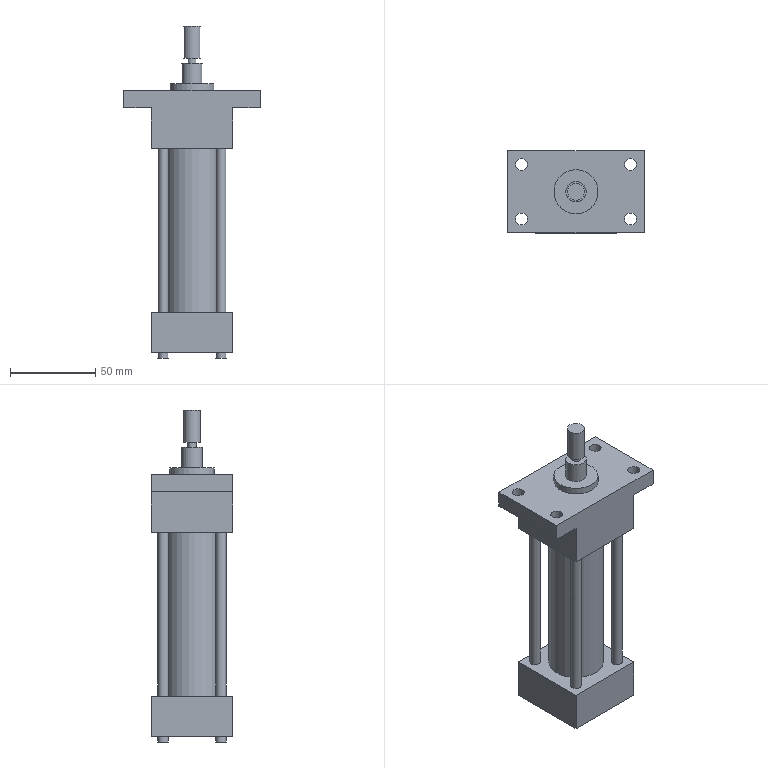Part | NX | features solid 2 | 1 solid | 48 faces | box 80 x 48 x 195 mm | volume 184667 mm3 | plane 28 | cylinder 20 | commonest cylinder face diameters 6 x8 7 x4 10 x3 5 x1 12 x1 26 x1
STEP:
#1=CARTESIAN_POINT('',(670.,59.,-219.));
#2=VERTEX_POINT('',#1);
#3=CARTESIAN_POINT('',(670.,75.,-219.));
#4=DIRECTION('',(0.,0.,1.));
#5=DIRECTION('',(0.,-1.,0.));
#6=AXIS2_PLACEMENT_3D('',#3,#4,#5);
#7=CIRCLE('',#6,16.);
#8=EDGE_CURVE('',#2,#2,#7,.T.);
#9=ORIENTED_EDGE('',*,*,#8,.F.);
#10=EDGE_LOOP('',(#9));
#11=FACE_BOUND('',#10,.T.);
#12=CARTESIAN_POINT('',(670.,59.,-315.));
#13=VERTEX_POINT('',#12);
#14=CARTESIAN_POINT('',(670.,75.,-315.));
#15=DIRECTION('',(0.,0.,1.));
#16=DIRECTION('',(0.,-1.,0.));
#17=AXIS2_PLACEMENT_3D('',#14,#15,#16);
#18=CIRCLE('',#17,16.);
#19=EDGE_CURVE('',#13,#13,#18,.F.);
#20=ORIENTED_EDGE('',*,*,#19,.F.);
#21=EDGE_LOOP('',(#20));
#22=FACE_BOUND('',#21,.T.);
#23=CARTESIAN_POINT('',(670.,75.,-339.));
#24=DIRECTION('',(0.,0.,1.));
#25=DIRECTION('',(0.,1.,0.));
#26=AXIS2_PLACEMENT_3D('',#23,#24,#25);
#27=CYLINDRICAL_SURFACE('',#26,16.);
#28=ADVANCED_FACE('',(#11,#22),#27,.T.);
#29=CARTESIAN_POINT('',(670.,81.,-169.));
#30=VERTEX_POINT('',#29);
#31=CARTESIAN_POINT('',(670.,75.,-169.));
#32=DIRECTION('',(0.,0.,-1.));
#33=DIRECTION('',(0.,1.,0.));
#34=AXIS2_PLACEMENT_3D('',#31,#32,#33);
#35=CIRCLE('',#34,6.);
#36=EDGE_CURVE('',#30,#30,#35,.T.);
#37=ORIENTED_EDGE('',*,*,#36,.F.);
#38=EDGE_LOOP('',(#37));
#39=FACE_BOUND('',#38,.T.);
#40=CARTESIAN_POINT('',(670.,77.5,-169.));
#41=VERTEX_POINT('',#40);
#42=CARTESIAN_POINT('',(670.,75.,-169.));
#43=DIRECTION('',(0.,0.,-1.));
#44=DIRECTION('',(0.,1.,0.));
#45=AXIS2_PLACEMENT_3D('',#42,#43,#44);
#46=CIRCLE('',#45,2.5);
#47=EDGE_CURVE('',#41,#41,#46,.T.);
#48=ORIENTED_EDGE('',*,*,#47,.T.);
#49=EDGE_LOOP('',(#48));
#50=FACE_BOUND('',#49,.T.);
#51=CARTESIAN_POINT('',(670.,75.,-169.));
#52=DIRECTION('',(0.,0.,1.));
#53=DIRECTION('',(0.,1.,0.));
#54=AXIS2_PLACEMENT_3D('',#51,#52,#53);
#55=PLANE('',#54);
#56=ADVANCED_FACE('',(#39,#50),#55,.T.);
#57=CARTESIAN_POINT('',(670.,88.,-181.));
#58=VERTEX_POINT('',#57);
#59=CARTESIAN_POINT('',(670.,75.,-181.));
#60=DIRECTION('',(0.,0.,-1.));
#61=DIRECTION('',(0.,1.,0.));
#62=AXIS2_PLACEMENT_3D('',#59,#60,#61);
#63=CIRCLE('',#62,13.);
#64=EDGE_CURVE('',#58,#58,#63,.T.);
#65=ORIENTED_EDGE('',*,*,#64,.F.);
#66=EDGE_LOOP('',(#65));
#67=FACE_BOUND('',#66,.T.);
#68=CARTESIAN_POINT('',(670.,81.,-181.));
#69=VERTEX_POINT('',#68);
#70=CARTESIAN_POINT('',(670.,75.,-181.));
#71=DIRECTION('',(0.,0.,-1.));
#72=DIRECTION('',(0.,1.,0.));
#73=AXIS2_PLACEMENT_3D('',#70,#71,#72);
#74=CIRCLE('',#73,6.);
#75=EDGE_CURVE('',#69,#69,#74,.F.);
#76=ORIENTED_EDGE('',*,*,#75,.F.);
#77=EDGE_LOOP('',(#76));
#78=FACE_BOUND('',#77,.T.);
#79=CARTESIAN_POINT('',(670.,75.,-181.));
#80=DIRECTION('',(0.,0.,1.));
#81=DIRECTION('',(0.,1.,0.));
#82=AXIS2_PLACEMENT_3D('',#79,#80,#81);
#83=PLANE('',#82);
#84=ADVANCED_FACE('',(#67,#78),#83,.T.);
#85=CARTESIAN_POINT('',(702.,62.5,-185.));
#86=VERTEX_POINT('',#85);
#87=CARTESIAN_POINT('',(702.,59.,-185.));
#88=DIRECTION('',(0.,0.,-1.));
#89=DIRECTION('',(0.,1.,0.));
#90=AXIS2_PLACEMENT_3D('',#87,#88,#89);
#91=CIRCLE('',#90,3.5);
#92=EDGE_CURVE('',#86,#86,#91,.T.);
#93=ORIENTED_EDGE('',*,*,#92,.T.);
#94=EDGE_LOOP('',(#93));
#95=FACE_BOUND('',#94,.T.);
#96=CARTESIAN_POINT('',(638.,94.5,-185.));
#97=VERTEX_POINT('',#96);
#98=CARTESIAN_POINT('',(638.,91.,-185.));
#99=DIRECTION('',(0.,0.,-1.));
#100=DIRECTION('',(0.,1.,0.));
#101=AXIS2_PLACEMENT_3D('',#98,#99,#100);
#102=CIRCLE('',#101,3.5);
#103=EDGE_CURVE('',#97,#97,#102,.T.);
#104=ORIENTED_EDGE('',*,*,#103,.T.);
#105=EDGE_LOOP('',(#104));
#106=FACE_BOUND('',#105,.T.);
#107=CARTESIAN_POINT('',(710.,51.,-185.));
#108=VERTEX_POINT('',#107);
#109=CARTESIAN_POINT('',(710.,99.,-185.));
#110=VERTEX_POINT('',#109);
#111=CARTESIAN_POINT('',(710.,51.,-185.));
#112=DIRECTION('',(0.,1.,0.));
#113=VECTOR('',#112,1000.);
#114=LINE('',#111,#113);
#115=EDGE_CURVE('',#108,#110,#114,.T.);
#116=ORIENTED_EDGE('',*,*,#115,.T.);
#117=CARTESIAN_POINT('',(630.,99.,-185.));
#118=VERTEX_POINT('',#117);
#119=CARTESIAN_POINT('',(630.,99.,-185.));
#120=DIRECTION('',(1.,0.,0.));
#121=VECTOR('',#120,1000.);
#122=LINE('',#119,#121);
#123=EDGE_CURVE('',#118,#110,#122,.T.);
#124=ORIENTED_EDGE('',*,*,#123,.F.);
#125=CARTESIAN_POINT('',(630.,51.,-185.));
#126=VERTEX_POINT('',#125);
#127=CARTESIAN_POINT('',(630.,51.,-185.));
#128=DIRECTION('',(0.,1.,0.));
#129=VECTOR('',#128,1000.);
#130=LINE('',#127,#129);
#131=EDGE_CURVE('',#126,#118,#130,.T.);
#132=ORIENTED_EDGE('',*,*,#131,.F.);
#133=CARTESIAN_POINT('',(694.,51.,-185.));
#134=DIRECTION('',(1.,0.,0.));
#135=VECTOR('',#134,1000.);
#136=LINE('',#133,#135);
#137=EDGE_CURVE('',#126,#108,#136,.T.);
#138=ORIENTED_EDGE('',*,*,#137,.T.);
#139=EDGE_LOOP('',(#116,#124,#132,#138));
#140=FACE_BOUND('',#139,.T.);
#141=CARTESIAN_POINT('',(638.,62.5,-185.));
#142=VERTEX_POINT('',#141);
#143=CARTESIAN_POINT('',(638.,59.,-185.));
#144=DIRECTION('',(0.,0.,-1.));
#145=DIRECTION('',(0.,1.,0.));
#146=AXIS2_PLACEMENT_3D('',#143,#144,#145);
#147=CIRCLE('',#146,3.5);
#148=EDGE_CURVE('',#142,#142,#147,.T.);
#149=ORIENTED_EDGE('',*,*,#148,.T.);
#150=EDGE_LOOP('',(#149));
#151=FACE_BOUND('',#150,.T.);
#152=CARTESIAN_POINT('',(702.,94.5,-185.));
#153=VERTEX_POINT('',#152);
#154=CARTESIAN_POINT('',(702.,91.,-185.));
#155=DIRECTION('',(0.,0.,-1.));
#156=DIRECTION('',(0.,1.,0.));
#157=AXIS2_PLACEMENT_3D('',#154,#155,#156);
#158=CIRCLE('',#157,3.5);
#159=EDGE_CURVE('',#153,#153,#158,.T.);
#160=ORIENTED_EDGE('',*,*,#159,.T.);
#161=EDGE_LOOP('',(#160));
#162=FACE_BOUND('',#161,.T.);
#163=CARTESIAN_POINT('',(670.,62.,-185.));
#164=VERTEX_POINT('',#163);
#165=CARTESIAN_POINT('',(670.,75.,-185.));
#166=DIRECTION('',(0.,0.,1.));
#167=DIRECTION('',(0.,-1.,0.));
#168=AXIS2_PLACEMENT_3D('',#165,#166,#167);
#169=CIRCLE('',#168,13.);
#170=EDGE_CURVE('',#164,#164,#169,.F.);
#171=ORIENTED_EDGE('',*,*,#170,.T.);
#172=EDGE_LOOP('',(#171));
#173=FACE_BOUND('',#172,.T.);
#174=CARTESIAN_POINT('',(710.,99.,-185.));
#175=DIRECTION('',(0.,0.,-1.));
#176=DIRECTION('',(0.,-1.,0.));
#177=AXIS2_PLACEMENT_3D('',#174,#175,#176);
#178=PLANE('',#177);
#179=ADVANCED_FACE('',(#95,#106,#140,#151,#162,#173),#178,.F.);
#180=CARTESIAN_POINT('',(646.,99.,-195.));
#181=VERTEX_POINT('',#180);
#182=CARTESIAN_POINT('',(646.,51.,-195.));
#183=VERTEX_POINT('',#182);
#184=CARTESIAN_POINT('',(646.,99.,-195.));
#185=DIRECTION('',(0.,-1.,0.));
#186=VECTOR('',#185,1000.);
#187=LINE('',#184,#186);
#188=EDGE_CURVE('',#181,#183,#187,.T.);
#189=ORIENTED_EDGE('',*,*,#188,.T.);
#190=CARTESIAN_POINT('',(630.,51.,-195.));
#191=VERTEX_POINT('',#190);
#192=CARTESIAN_POINT('',(694.,51.,-195.));
#193=DIRECTION('',(1.,0.,0.));
#194=VECTOR('',#193,1000.);
#195=LINE('',#192,#194);
#196=EDGE_CURVE('',#191,#183,#195,.T.);
#197=ORIENTED_EDGE('',*,*,#196,.F.);
#198=CARTESIAN_POINT('',(630.,99.,-195.));
#199=VERTEX_POINT('',#198);
#200=CARTESIAN_POINT('',(630.,51.,-195.));
#201=DIRECTION('',(0.,1.,0.));
#202=VECTOR('',#201,1000.);
#203=LINE('',#200,#202);
#204=EDGE_CURVE('',#191,#199,#203,.T.);
#205=ORIENTED_EDGE('',*,*,#204,.T.);
#206=CARTESIAN_POINT('',(630.,99.,-195.));
#207=DIRECTION('',(1.,0.,0.));
#208=VECTOR('',#207,1000.);
#209=LINE('',#206,#208);
#210=EDGE_CURVE('',#199,#181,#209,.T.);
#211=ORIENTED_EDGE('',*,*,#210,.T.);
#212=EDGE_LOOP('',(#189,#197,#205,#211));
#213=FACE_BOUND('',#212,.T.);
#214=CARTESIAN_POINT('',(638.,94.5,-195.));
#215=VERTEX_POINT('',#214);
#216=CARTESIAN_POINT('',(638.,91.,-195.));
#217=DIRECTION('',(0.,0.,-1.));
#218=DIRECTION('',(0.,1.,0.));
#219=AXIS2_PLACEMENT_3D('',#216,#217,#218);
#220=CIRCLE('',#219,3.5);
#221=EDGE_CURVE('',#215,#215,#220,.T.);
#222=ORIENTED_EDGE('',*,*,#221,.F.);
#223=EDGE_LOOP('',(#222));
#224=FACE_BOUND('',#223,.T.);
#225=CARTESIAN_POINT('',(638.,62.5,-195.));
#226=VERTEX_POINT('',#225);
#227=CARTESIAN_POINT('',(638.,59.,-195.));
#228=DIRECTION('',(0.,0.,-1.));
#229=DIRECTION('',(0.,1.,0.));
#230=AXIS2_PLACEMENT_3D('',#227,#228,#229);
#231=CIRCLE('',#230,3.5);
#232=EDGE_CURVE('',#226,#226,#231,.T.);
#233=ORIENTED_EDGE('',*,*,#232,.F.);
#234=EDGE_LOOP('',(#233));
#235=FACE_BOUND('',#234,.T.);
#236=CARTESIAN_POINT('',(710.,99.,-195.));
#237=DIRECTION('',(0.,0.,-1.));
#238=DIRECTION('',(0.,-1.,0.));
#239=AXIS2_PLACEMENT_3D('',#236,#237,#238);
#240=PLANE('',#239);
#241=ADVANCED_FACE('',(#213,#224,#235),#240,.T.);
#242=ORIENTED_EDGE('',*,*,#115,.F.);
#243=CARTESIAN_POINT('',(710.,51.,-195.));
#244=VERTEX_POINT('',#243);
#245=CARTESIAN_POINT('',(710.,51.,-195.));
#246=DIRECTION('',(0.,0.,1.));
#247=VECTOR('',#246,1000.);
#248=LINE('',#245,#247);
#249=EDGE_CURVE('',#244,#108,#248,.T.);
#250=ORIENTED_EDGE('',*,*,#249,.F.);
#251=CARTESIAN_POINT('',(710.,99.,-195.));
#252=VERTEX_POINT('',#251);
#253=CARTESIAN_POINT('',(710.,51.,-195.));
#254=DIRECTION('',(0.,1.,0.));
#255=VECTOR('',#254,1000.);
#256=LINE('',#253,#255);
#257=EDGE_CURVE('',#244,#252,#256,.T.);
#258=ORIENTED_EDGE('',*,*,#257,.T.);
#259=CARTESIAN_POINT('',(710.,99.,-195.));
#260=DIRECTION('',(0.,0.,1.));
#261=VECTOR('',#260,1000.);
#262=LINE('',#259,#261);
#263=EDGE_CURVE('',#252,#110,#262,.T.);
#264=ORIENTED_EDGE('',*,*,#263,.T.);
#265=EDGE_LOOP('',(#242,#250,#258,#264));
#266=FACE_BOUND('',#265,.T.);
#267=CARTESIAN_POINT('',(710.,51.,-195.));
#268=DIRECTION('',(-1.,0.,0.));
#269=DIRECTION('',(0.,0.,-1.));
#270=AXIS2_PLACEMENT_3D('',#267,#268,#269);
#271=PLANE('',#270);
#272=ADVANCED_FACE('',(#266),#271,.F.);
#273=CARTESIAN_POINT('',(665.,99.,-207.));
#274=VERTEX_POINT('',#273);
#275=CARTESIAN_POINT('',(670.,99.,-207.));
#276=DIRECTION('',(0.,1.,0.));
#277=DIRECTION('',(-1.,0.,0.));
#278=AXIS2_PLACEMENT_3D('',#275,#276,#277);
#279=CIRCLE('',#278,5.);
#280=EDGE_CURVE('',#274,#274,#279,.T.);
#281=ORIENTED_EDGE('',*,*,#280,.F.);
#282=EDGE_LOOP('',(#281));
#283=FACE_BOUND('',#282,.T.);
#284=ORIENTED_EDGE('',*,*,#123,.T.);
#285=ORIENTED_EDGE('',*,*,#263,.F.);
#286=CARTESIAN_POINT('',(694.,99.,-195.));
#287=VERTEX_POINT('',#286);
#288=CARTESIAN_POINT('',(630.,99.,-195.));
#289=DIRECTION('',(1.,0.,0.));
#290=VECTOR('',#289,1000.);
#291=LINE('',#288,#290);
#292=EDGE_CURVE('',#287,#252,#291,.T.);
#293=ORIENTED_EDGE('',*,*,#292,.F.);
#294=CARTESIAN_POINT('',(694.,99.,-219.));
#295=VERTEX_POINT('',#294);
#296=CARTESIAN_POINT('',(694.,99.,-219.));
#297=DIRECTION('',(0.,0.,1.));
#298=VECTOR('',#297,1000.);
#299=LINE('',#296,#298);
#300=EDGE_CURVE('',#295,#287,#299,.T.);
#301=ORIENTED_EDGE('',*,*,#300,.F.);
#302=CARTESIAN_POINT('',(646.,99.,-219.));
#303=VERTEX_POINT('',#302);
#304=CARTESIAN_POINT('',(694.,99.,-219.));
#305=DIRECTION('',(-1.,0.,0.));
#306=VECTOR('',#305,1000.);
#307=LINE('',#304,#306);
#308=EDGE_CURVE('',#295,#303,#307,.T.);
#309=ORIENTED_EDGE('',*,*,#308,.T.);
#310=CARTESIAN_POINT('',(646.,99.,-219.));
#311=DIRECTION('',(0.,0.,1.));
#312=VECTOR('',#311,1000.);
#313=LINE('',#310,#312);
#314=EDGE_CURVE('',#303,#181,#313,.T.);
#315=ORIENTED_EDGE('',*,*,#314,.T.);
#316=ORIENTED_EDGE('',*,*,#210,.F.);
#317=CARTESIAN_POINT('',(630.,99.,-195.));
#318=DIRECTION('',(0.,0.,1.));
#319=VECTOR('',#318,1000.);
#320=LINE('',#317,#319);
#321=EDGE_CURVE('',#199,#118,#320,.T.);
#322=ORIENTED_EDGE('',*,*,#321,.T.);
#323=EDGE_LOOP('',(#284,#285,#293,#301,#309,#315,#316,#322));
#324=FACE_BOUND('',#323,.T.);
#325=CARTESIAN_POINT('',(630.,99.,-195.));
#326=DIRECTION('',(0.,1.,0.));
#327=DIRECTION('',(1.,0.,0.));
#328=AXIS2_PLACEMENT_3D('',#325,#326,#327);
#329=PLANE('',#328);
#330=ADVANCED_FACE('',(#283,#324),#329,.T.);
#331=ORIENTED_EDGE('',*,*,#131,.T.);
#332=ORIENTED_EDGE('',*,*,#321,.F.);
#333=ORIENTED_EDGE('',*,*,#204,.F.);
#334=CARTESIAN_POINT('',(630.,51.,-195.));
#335=DIRECTION('',(0.,0.,1.));
#336=VECTOR('',#335,1000.);
#337=LINE('',#334,#336);
#338=EDGE_CURVE('',#191,#126,#337,.T.);
#339=ORIENTED_EDGE('',*,*,#338,.T.);
#340=EDGE_LOOP('',(#331,#332,#333,#339));
#341=FACE_BOUND('',#340,.T.);
#342=CARTESIAN_POINT('',(630.,51.,-195.));
#343=DIRECTION('',(-1.,0.,0.));
#344=DIRECTION('',(0.,0.,-1.));
#345=AXIS2_PLACEMENT_3D('',#342,#343,#344);
#346=PLANE('',#345);
#347=ADVANCED_FACE('',(#341),#346,.T.);
#348=ORIENTED_EDGE('',*,*,#221,.T.);
#349=EDGE_LOOP('',(#348));
#350=FACE_BOUND('',#349,.T.);
#351=ORIENTED_EDGE('',*,*,#103,.F.);
#352=EDGE_LOOP('',(#351));
#353=FACE_BOUND('',#352,.T.);
#354=CARTESIAN_POINT('',(638.,91.,-195.));
#355=DIRECTION('',(0.,0.,1.));
#356=DIRECTION('',(0.,1.,0.));
#357=AXIS2_PLACEMENT_3D('',#354,#355,#356);
#358=CYLINDRICAL_SURFACE('',#357,3.5);
#359=ADVANCED_FACE('',(#350,#353),#358,.F.);
#360=ORIENTED_EDGE('',*,*,#137,.F.);
#361=ORIENTED_EDGE('',*,*,#338,.F.);
#362=ORIENTED_EDGE('',*,*,#196,.T.);
#363=CARTESIAN_POINT('',(646.,51.,-219.));
#364=VERTEX_POINT('',#363);
#365=CARTESIAN_POINT('',(646.,51.,-219.));
#366=DIRECTION('',(0.,0.,1.));
#367=VECTOR('',#366,1000.);
#368=LINE('',#365,#367);
#369=EDGE_CURVE('',#364,#183,#368,.T.);
#370=ORIENTED_EDGE('',*,*,#369,.F.);
#371=CARTESIAN_POINT('',(694.,51.,-219.));
#372=VERTEX_POINT('',#371);
#373=CARTESIAN_POINT('',(646.,51.,-219.));
#374=DIRECTION('',(1.,0.,0.));
#375=VECTOR('',#374,1000.);
#376=LINE('',#373,#375);
#377=EDGE_CURVE('',#364,#372,#376,.T.);
#378=ORIENTED_EDGE('',*,*,#377,.T.);
#379=CARTESIAN_POINT('',(694.,51.,-195.));
#380=VERTEX_POINT('',#379);
#381=CARTESIAN_POINT('',(694.,51.,-219.));
#382=DIRECTION('',(0.,0.,1.));
#383=VECTOR('',#382,1000.);
#384=LINE('',#381,#383);
#385=EDGE_CURVE('',#372,#380,#384,.T.);
#386=ORIENTED_EDGE('',*,*,#385,.T.);
#387=CARTESIAN_POINT('',(694.,51.,-195.));
#388=DIRECTION('',(1.,0.,0.));
#389=VECTOR('',#388,1000.);
#390=LINE('',#387,#389);
#391=EDGE_CURVE('',#380,#244,#390,.T.);
#392=ORIENTED_EDGE('',*,*,#391,.T.);
#393=ORIENTED_EDGE('',*,*,#249,.T.);
#394=EDGE_LOOP('',(#360,#361,#362,#370,#378,#386,#392,#393));
#395=FACE_BOUND('',#394,.T.);
#396=CARTESIAN_POINT('',(694.,51.,-195.));
#397=DIRECTION('',(0.,1.,0.));
#398=DIRECTION('',(0.,0.,-1.));
#399=AXIS2_PLACEMENT_3D('',#396,#397,#398);
#400=PLANE('',#399);
#401=ADVANCED_FACE('',(#395),#400,.F.);
#402=ORIENTED_EDGE('',*,*,#232,.T.);
#403=EDGE_LOOP('',(#402));
#404=FACE_BOUND('',#403,.T.);
#405=ORIENTED_EDGE('',*,*,#148,.F.);
#406=EDGE_LOOP('',(#405));
#407=FACE_BOUND('',#406,.T.);
#408=CARTESIAN_POINT('',(638.,59.,-195.));
#409=DIRECTION('',(0.,0.,1.));
#410=DIRECTION('',(0.,1.,0.));
#411=AXIS2_PLACEMENT_3D('',#408,#409,#410);
#412=CYLINDRICAL_SURFACE('',#411,3.5);
#413=ADVANCED_FACE('',(#404,#407),#412,.F.);
#414=CARTESIAN_POINT('',(702.,94.5,-195.));
#415=VERTEX_POINT('',#414);
#416=CARTESIAN_POINT('',(702.,91.,-195.));
#417=DIRECTION('',(0.,0.,-1.));
#418=DIRECTION('',(0.,1.,0.));
#419=AXIS2_PLACEMENT_3D('',#416,#417,#418);
#420=CIRCLE('',#419,3.5);
#421=EDGE_CURVE('',#415,#415,#420,.T.);
#422=ORIENTED_EDGE('',*,*,#421,.T.);
#423=EDGE_LOOP('',(#422));
#424=FACE_BOUND('',#423,.T.);
#425=ORIENTED_EDGE('',*,*,#159,.F.);
#426=EDGE_LOOP('',(#425));
#427=FACE_BOUND('',#426,.T.);
#428=CARTESIAN_POINT('',(702.,91.,-195.));
#429=DIRECTION('',(0.,0.,1.));
#430=DIRECTION('',(0.,1.,0.));
#431=AXIS2_PLACEMENT_3D('',#428,#429,#430);
#432=CYLINDRICAL_SURFACE('',#431,3.5);
#433=ADVANCED_FACE('',(#424,#427),#432,.F.);
#434=CARTESIAN_POINT('',(702.,62.5,-195.));
#435=VERTEX_POINT('',#434);
#436=CARTESIAN_POINT('',(702.,59.,-195.));
#437=DIRECTION('',(0.,0.,-1.));
#438=DIRECTION('',(0.,1.,0.));
#439=AXIS2_PLACEMENT_3D('',#436,#437,#438);
#440=CIRCLE('',#439,3.5);
#441=EDGE_CURVE('',#435,#435,#440,.T.);
#442=ORIENTED_EDGE('',*,*,#441,.T.);
#443=EDGE_LOOP('',(#442));
#444=FACE_BOUND('',#443,.T.);
#445=ORIENTED_EDGE('',*,*,#92,.F.);
#446=EDGE_LOOP('',(#445));
#447=FACE_BOUND('',#446,.T.);
#448=CARTESIAN_POINT('',(702.,59.,-195.));
#449=DIRECTION('',(0.,0.,1.));
#450=DIRECTION('',(0.,1.,0.));
#451=AXIS2_PLACEMENT_3D('',#448,#449,#450);
#452=CYLINDRICAL_SURFACE('',#451,3.5);
#453=ADVANCED_FACE('',(#444,#447),#452,.F.);
#454=CARTESIAN_POINT('',(694.,51.,-195.));
#455=DIRECTION('',(0.,1.,0.));
#456=VECTOR('',#455,1000.);
#457=LINE('',#454,#456);
#458=EDGE_CURVE('',#380,#287,#457,.T.);
#459=ORIENTED_EDGE('',*,*,#458,.T.);
#460=ORIENTED_EDGE('',*,*,#292,.T.);
#461=ORIENTED_EDGE('',*,*,#257,.F.);
#462=ORIENTED_EDGE('',*,*,#391,.F.);
#463=EDGE_LOOP('',(#459,#460,#461,#462));
#464=FACE_BOUND('',#463,.T.);
#465=ORIENTED_EDGE('',*,*,#421,.F.);
#466=EDGE_LOOP('',(#465));
#467=FACE_BOUND('',#466,.T.);
#468=ORIENTED_EDGE('',*,*,#441,.F.);
#469=EDGE_LOOP('',(#468));
#470=FACE_BOUND('',#469,.T.);
#471=CARTESIAN_POINT('',(710.,99.,-195.));
#472=DIRECTION('',(0.,0.,-1.));
#473=DIRECTION('',(0.,-1.,0.));
#474=AXIS2_PLACEMENT_3D('',#471,#472,#473);
#475=PLANE('',#474);
#476=ADVANCED_FACE('',(#464,#467,#470),#475,.T.);
#477=ORIENTED_EDGE('',*,*,#458,.F.);
#478=ORIENTED_EDGE('',*,*,#385,.F.);
#479=CARTESIAN_POINT('',(694.,51.,-219.));
#480=DIRECTION('',(0.,1.,0.));
#481=VECTOR('',#480,1000.);
#482=LINE('',#479,#481);
#483=EDGE_CURVE('',#372,#295,#482,.T.);
#484=ORIENTED_EDGE('',*,*,#483,.T.);
#485=ORIENTED_EDGE('',*,*,#300,.T.);
#486=EDGE_LOOP('',(#477,#478,#484,#485));
#487=FACE_BOUND('',#486,.T.);
#488=CARTESIAN_POINT('',(694.,51.,-219.));
#489=DIRECTION('',(-1.,0.,0.));
#490=DIRECTION('',(0.,0.,-1.));
#491=AXIS2_PLACEMENT_3D('',#488,#489,#490);
#492=PLANE('',#491);
#493=ADVANCED_FACE('',(#487),#492,.F.);
#494=ORIENTED_EDGE('',*,*,#188,.F.);
#495=ORIENTED_EDGE('',*,*,#314,.F.);
#496=CARTESIAN_POINT('',(646.,99.,-219.));
#497=DIRECTION('',(0.,-1.,0.));
#498=VECTOR('',#497,1000.);
#499=LINE('',#496,#498);
#500=EDGE_CURVE('',#303,#364,#499,.T.);
#501=ORIENTED_EDGE('',*,*,#500,.T.);
#502=ORIENTED_EDGE('',*,*,#369,.T.);
#503=EDGE_LOOP('',(#494,#495,#501,#502));
#504=FACE_BOUND('',#503,.T.);
#505=CARTESIAN_POINT('',(646.,99.,-219.));
#506=DIRECTION('',(1.,0.,0.));
#507=DIRECTION('',(0.,0.,1.));
#508=AXIS2_PLACEMENT_3D('',#505,#506,#507);
#509=PLANE('',#508);
#510=ADVANCED_FACE('',(#504),#509,.F.);
#511=CARTESIAN_POINT('',(687.,89.,-219.));
#512=VERTEX_POINT('',#511);
#513=CARTESIAN_POINT('',(687.,92.,-219.));
#514=DIRECTION('',(0.,0.,1.));
#515=DIRECTION('',(0.,-1.,0.));
#516=AXIS2_PLACEMENT_3D('',#513,#514,#515);
#517=CIRCLE('',#516,3.);
#518=EDGE_CURVE('',#512,#512,#517,.T.);
#519=ORIENTED_EDGE('',*,*,#518,.T.);
#520=EDGE_LOOP('',(#519));
#521=FACE_BOUND('',#520,.T.);
#522=CARTESIAN_POINT('',(687.,55.,-219.));
#523=VERTEX_POINT('',#522);
#524=CARTESIAN_POINT('',(687.,58.,-219.));
#525=DIRECTION('',(0.,0.,1.));
#526=DIRECTION('',(0.,-1.,0.));
#527=AXIS2_PLACEMENT_3D('',#524,#525,#526);
#528=CIRCLE('',#527,3.);
#529=EDGE_CURVE('',#523,#523,#528,.T.);
#530=ORIENTED_EDGE('',*,*,#529,.T.);
#531=EDGE_LOOP('',(#530));
#532=FACE_BOUND('',#531,.T.);
#533=CARTESIAN_POINT('',(653.,55.,-219.));
#534=VERTEX_POINT('',#533);
#535=CARTESIAN_POINT('',(653.,58.,-219.));
#536=DIRECTION('',(0.,0.,1.));
#537=DIRECTION('',(0.,-1.,0.));
#538=AXIS2_PLACEMENT_3D('',#535,#536,#537);
#539=CIRCLE('',#538,3.);
#540=EDGE_CURVE('',#534,#534,#539,.T.);
#541=ORIENTED_EDGE('',*,*,#540,.T.);
#542=EDGE_LOOP('',(#541));
#543=FACE_BOUND('',#542,.T.);
#544=CARTESIAN_POINT('',(653.,89.,-219.));
#545=VERTEX_POINT('',#544);
#546=CARTESIAN_POINT('',(653.,92.,-219.));
#547=DIRECTION('',(0.,0.,1.));
#548=DIRECTION('',(0.,-1.,0.));
#549=AXIS2_PLACEMENT_3D('',#546,#547,#548);
#550=CIRCLE('',#549,3.);
#551=EDGE_CURVE('',#545,#545,#550,.T.);
#552=ORIENTED_EDGE('',*,*,#551,.T.);
#553=EDGE_LOOP('',(#552));
#554=FACE_BOUND('',#553,.T.);
#555=ORIENTED_EDGE('',*,*,#8,.T.);
#556=EDGE_LOOP('',(#555));
#557=FACE_BOUND('',#556,.T.);
#558=ORIENTED_EDGE('',*,*,#377,.F.);
#559=ORIENTED_EDGE('',*,*,#500,.F.);
#560=ORIENTED_EDGE('',*,*,#308,.F.);
#561=ORIENTED_EDGE('',*,*,#483,.F.);
#562=EDGE_LOOP('',(#558,#559,#560,#561));
#563=FACE_BOUND('',#562,.T.);
#564=CARTESIAN_POINT('',(694.,51.,-219.));
#565=DIRECTION('',(0.,0.,-1.));
#566=DIRECTION('',(0.,-1.,0.));
#567=AXIS2_PLACEMENT_3D('',#564,#565,#566);
#568=PLANE('',#567);
#569=ADVANCED_FACE('',(#521,#532,#543,#554,#557,#563),#568,.T.);
#570=ORIENTED_EDGE('',*,*,#64,.T.);
#571=EDGE_LOOP('',(#570));
#572=FACE_BOUND('',#571,.T.);
#573=ORIENTED_EDGE('',*,*,#170,.F.);
#574=EDGE_LOOP('',(#573));
#575=FACE_BOUND('',#574,.T.);
#576=CARTESIAN_POINT('',(670.,75.,-181.));
#577=DIRECTION('',(0.,0.,-1.));
#578=DIRECTION('',(0.,-1.,0.));
#579=AXIS2_PLACEMENT_3D('',#576,#577,#578);
#580=CYLINDRICAL_SURFACE('',#579,13.);
#581=ADVANCED_FACE('',(#572,#575),#580,.T.);
#582=ORIENTED_EDGE('',*,*,#75,.T.);
#583=EDGE_LOOP('',(#582));
#584=FACE_BOUND('',#583,.T.);
#585=ORIENTED_EDGE('',*,*,#36,.T.);
#586=EDGE_LOOP('',(#585));
#587=FACE_BOUND('',#586,.T.);
#588=CARTESIAN_POINT('',(670.,75.,-169.));
#589=DIRECTION('',(0.,0.,-1.));
#590=DIRECTION('',(0.,-1.,0.));
#591=AXIS2_PLACEMENT_3D('',#588,#589,#590);
#592=CYLINDRICAL_SURFACE('',#591,6.);
#593=ADVANCED_FACE('',(#584,#587),#592,.T.);
#594=CARTESIAN_POINT('',(646.,51.,-315.));
#595=VERTEX_POINT('',#594);
#596=CARTESIAN_POINT('',(694.,51.,-315.));
#597=VERTEX_POINT('',#596);
#598=CARTESIAN_POINT('',(646.,51.,-315.));
#599=DIRECTION('',(1.,0.,0.));
#600=VECTOR('',#599,1000.);
#601=LINE('',#598,#600);
#602=EDGE_CURVE('',#595,#597,#601,.T.);
#603=ORIENTED_EDGE('',*,*,#602,.F.);
#604=CARTESIAN_POINT('',(646.,51.,-339.));
#605=VERTEX_POINT('',#604);
#606=CARTESIAN_POINT('',(646.,51.,-339.));
#607=DIRECTION('',(0.,0.,1.));
#608=VECTOR('',#607,1000.);
#609=LINE('',#606,#608);
#610=EDGE_CURVE('',#605,#595,#609,.T.);
#611=ORIENTED_EDGE('',*,*,#610,.F.);
#612=CARTESIAN_POINT('',(694.,51.,-339.));
#613=VERTEX_POINT('',#612);
#614=CARTESIAN_POINT('',(646.,51.,-339.));
#615=DIRECTION('',(1.,0.,0.));
#616=VECTOR('',#615,1000.);
#617=LINE('',#614,#616);
#618=EDGE_CURVE('',#605,#613,#617,.T.);
#619=ORIENTED_EDGE('',*,*,#618,.T.);
#620=CARTESIAN_POINT('',(694.,51.,-339.));
#621=DIRECTION('',(0.,0.,1.));
#622=VECTOR('',#621,1000.);
#623=LINE('',#620,#622);
#624=EDGE_CURVE('',#613,#597,#623,.T.);
#625=ORIENTED_EDGE('',*,*,#624,.T.);
#626=EDGE_LOOP('',(#603,#611,#619,#625));
#627=FACE_BOUND('',#626,.T.);
#628=CARTESIAN_POINT('',(646.,51.,-339.));
#629=DIRECTION('',(0.,1.,0.));
#630=DIRECTION('',(0.,0.,-1.));
#631=AXIS2_PLACEMENT_3D('',#628,#629,#630);
#632=PLANE('',#631);
#633=ADVANCED_FACE('',(#627),#632,.F.);
#634=CARTESIAN_POINT('',(694.,99.,-315.));
#635=VERTEX_POINT('',#634);
#636=CARTESIAN_POINT('',(694.,51.,-315.));
#637=DIRECTION('',(0.,1.,0.));
#638=VECTOR('',#637,1000.);
#639=LINE('',#636,#638);
#640=EDGE_CURVE('',#597,#635,#639,.T.);
#641=ORIENTED_EDGE('',*,*,#640,.F.);
#642=ORIENTED_EDGE('',*,*,#624,.F.);
#643=CARTESIAN_POINT('',(694.,99.,-339.));
#644=VERTEX_POINT('',#643);
#645=CARTESIAN_POINT('',(694.,51.,-339.));
#646=DIRECTION('',(0.,1.,0.));
#647=VECTOR('',#646,1000.);
#648=LINE('',#645,#647);
#649=EDGE_CURVE('',#613,#644,#648,.T.);
#650=ORIENTED_EDGE('',*,*,#649,.T.);
#651=CARTESIAN_POINT('',(694.,99.,-339.));
#652=DIRECTION('',(0.,0.,1.));
#653=VECTOR('',#652,1000.);
#654=LINE('',#651,#653);
#655=EDGE_CURVE('',#644,#635,#654,.T.);
#656=ORIENTED_EDGE('',*,*,#655,.T.);
#657=EDGE_LOOP('',(#641,#642,#650,#656));
#658=FACE_BOUND('',#657,.T.);
#659=CARTESIAN_POINT('',(694.,51.,-339.));
#660=DIRECTION('',(-1.,0.,0.));
#661=DIRECTION('',(0.,0.,-1.));
#662=AXIS2_PLACEMENT_3D('',#659,#660,#661);
#663=PLANE('',#662);
#664=ADVANCED_FACE('',(#658),#663,.F.);
#665=CARTESIAN_POINT('',(665.,99.,-327.));
#666=VERTEX_POINT('',#665);
#667=CARTESIAN_POINT('',(670.,99.,-327.));
#668=DIRECTION('',(0.,1.,0.));
#669=DIRECTION('',(-1.,0.,0.));
#670=AXIS2_PLACEMENT_3D('',#667,#668,#669);
#671=CIRCLE('',#670,5.);
#672=EDGE_CURVE('',#666,#666,#671,.T.);
#673=ORIENTED_EDGE('',*,*,#672,.F.);
#674=EDGE_LOOP('',(#673));
#675=FACE_BOUND('',#674,.T.);
#676=CARTESIAN_POINT('',(646.,99.,-315.));
#677=VERTEX_POINT('',#676);
#678=CARTESIAN_POINT('',(694.,99.,-315.));
#679=DIRECTION('',(-1.,0.,0.));
#680=VECTOR('',#679,1000.);
#681=LINE('',#678,#680);
#682=EDGE_CURVE('',#635,#677,#681,.T.);
#683=ORIENTED_EDGE('',*,*,#682,.F.);
#684=ORIENTED_EDGE('',*,*,#655,.F.);
#685=CARTESIAN_POINT('',(646.,99.,-339.));
#686=VERTEX_POINT('',#685);
#687=CARTESIAN_POINT('',(694.,99.,-339.));
#688=DIRECTION('',(-1.,0.,0.));
#689=VECTOR('',#688,1000.);
#690=LINE('',#687,#689);
#691=EDGE_CURVE('',#644,#686,#690,.T.);
#692=ORIENTED_EDGE('',*,*,#691,.T.);
#693=CARTESIAN_POINT('',(646.,99.,-339.));
#694=DIRECTION('',(0.,0.,1.));
#695=VECTOR('',#694,1000.);
#696=LINE('',#693,#695);
#697=EDGE_CURVE('',#686,#677,#696,.T.);
#698=ORIENTED_EDGE('',*,*,#697,.T.);
#699=EDGE_LOOP('',(#683,#684,#692,#698));
#700=FACE_BOUND('',#699,.T.);
#701=CARTESIAN_POINT('',(694.,99.,-339.));
#702=DIRECTION('',(0.,-1.,0.));
#703=DIRECTION('',(-1.,0.,0.));
#704=AXIS2_PLACEMENT_3D('',#701,#702,#703);
#705=PLANE('',#704);
#706=ADVANCED_FACE('',(#675,#700),#705,.F.);
#707=CARTESIAN_POINT('',(646.,99.,-315.));
#708=DIRECTION('',(0.,-1.,0.));
#709=VECTOR('',#708,1000.);
#710=LINE('',#707,#709);
#711=EDGE_CURVE('',#677,#595,#710,.T.);
#712=ORIENTED_EDGE('',*,*,#711,.F.);
#713=ORIENTED_EDGE('',*,*,#697,.F.);
#714=CARTESIAN_POINT('',(646.,99.,-339.));
#715=DIRECTION('',(0.,-1.,0.));
#716=VECTOR('',#715,1000.);
#717=LINE('',#714,#716);
#718=EDGE_CURVE('',#686,#605,#717,.T.);
#719=ORIENTED_EDGE('',*,*,#718,.T.);
#720=ORIENTED_EDGE('',*,*,#610,.T.);
#721=EDGE_LOOP('',(#712,#713,#719,#720));
#722=FACE_BOUND('',#721,.T.);
#723=CARTESIAN_POINT('',(646.,99.,-339.));
#724=DIRECTION('',(1.,0.,0.));
#725=DIRECTION('',(0.,0.,1.));
#726=AXIS2_PLACEMENT_3D('',#723,#724,#725);
#727=PLANE('',#726);
#728=ADVANCED_FACE('',(#722),#727,.F.);
#729=CARTESIAN_POINT('',(687.,89.,-315.));
#730=VERTEX_POINT('',#729);
#731=CARTESIAN_POINT('',(687.,92.,-315.));
#732=DIRECTION('',(0.,0.,1.));
#733=DIRECTION('',(0.,-1.,0.));
#734=AXIS2_PLACEMENT_3D('',#731,#732,#733);
#735=CIRCLE('',#734,3.);
#736=EDGE_CURVE('',#730,#730,#735,.T.);
#737=ORIENTED_EDGE('',*,*,#736,.F.);
#738=EDGE_LOOP('',(#737));
#739=FACE_BOUND('',#738,.T.);
#740=CARTESIAN_POINT('',(687.,55.,-315.));
#741=VERTEX_POINT('',#740);
#742=CARTESIAN_POINT('',(687.,58.,-315.));
#743=DIRECTION('',(0.,0.,1.));
#744=DIRECTION('',(0.,-1.,0.));
#745=AXIS2_PLACEMENT_3D('',#742,#743,#744);
#746=CIRCLE('',#745,3.);
#747=EDGE_CURVE('',#741,#741,#746,.T.);
#748=ORIENTED_EDGE('',*,*,#747,.F.);
#749=EDGE_LOOP('',(#748));
#750=FACE_BOUND('',#749,.T.);
#751=CARTESIAN_POINT('',(653.,55.,-315.));
#752=VERTEX_POINT('',#751);
#753=CARTESIAN_POINT('',(653.,58.,-315.));
#754=DIRECTION('',(0.,0.,1.));
#755=DIRECTION('',(0.,-1.,0.));
#756=AXIS2_PLACEMENT_3D('',#753,#754,#755);
#757=CIRCLE('',#756,3.);
#758=EDGE_CURVE('',#752,#752,#757,.T.);
#759=ORIENTED_EDGE('',*,*,#758,.F.);
#760=EDGE_LOOP('',(#759));
#761=FACE_BOUND('',#760,.T.);
#762=CARTESIAN_POINT('',(653.,89.,-315.));
#763=VERTEX_POINT('',#762);
#764=CARTESIAN_POINT('',(653.,92.,-315.));
#765=DIRECTION('',(0.,0.,1.));
#766=DIRECTION('',(0.,-1.,0.));
#767=AXIS2_PLACEMENT_3D('',#764,#765,#766);
#768=CIRCLE('',#767,3.);
#769=EDGE_CURVE('',#763,#763,#768,.T.);
#770=ORIENTED_EDGE('',*,*,#769,.F.);
#771=EDGE_LOOP('',(#770));
#772=FACE_BOUND('',#771,.T.);
#773=ORIENTED_EDGE('',*,*,#19,.T.);
#774=EDGE_LOOP('',(#773));
#775=FACE_BOUND('',#774,.T.);
#776=ORIENTED_EDGE('',*,*,#602,.T.);
#777=ORIENTED_EDGE('',*,*,#640,.T.);
#778=ORIENTED_EDGE('',*,*,#682,.T.);
#779=ORIENTED_EDGE('',*,*,#711,.T.);
#780=EDGE_LOOP('',(#776,#777,#778,#779));
#781=FACE_BOUND('',#780,.T.);
#782=CARTESIAN_POINT('',(694.,51.,-315.));
#783=DIRECTION('',(0.,0.,-1.));
#784=DIRECTION('',(0.,-1.,0.));
#785=AXIS2_PLACEMENT_3D('',#782,#783,#784);
#786=PLANE('',#785);
#787=ADVANCED_FACE('',(#739,#750,#761,#772,#775,#781),#786,.F.);
#788=CARTESIAN_POINT('',(687.,95.,-339.));
#789=VERTEX_POINT('',#788);
#790=CARTESIAN_POINT('',(687.,92.,-339.));
#791=DIRECTION('',(0.,0.,-1.));
#792=DIRECTION('',(0.,1.,0.));
#793=AXIS2_PLACEMENT_3D('',#790,#791,#792);
#794=CIRCLE('',#793,3.);
#795=EDGE_CURVE('',#789,#789,#794,.T.);
#796=ORIENTED_EDGE('',*,*,#795,.F.);
#797=EDGE_LOOP('',(#796));
#798=FACE_BOUND('',#797,.T.);
#799=CARTESIAN_POINT('',(687.,61.,-339.));
#800=VERTEX_POINT('',#799);
#801=CARTESIAN_POINT('',(687.,58.,-339.));
#802=DIRECTION('',(0.,0.,-1.));
#803=DIRECTION('',(0.,1.,0.));
#804=AXIS2_PLACEMENT_3D('',#801,#802,#803);
#805=CIRCLE('',#804,3.);
#806=EDGE_CURVE('',#800,#800,#805,.T.);
#807=ORIENTED_EDGE('',*,*,#806,.F.);
#808=EDGE_LOOP('',(#807));
#809=FACE_BOUND('',#808,.T.);
#810=CARTESIAN_POINT('',(653.,61.,-339.));
#811=VERTEX_POINT('',#810);
#812=CARTESIAN_POINT('',(653.,58.,-339.));
#813=DIRECTION('',(0.,0.,-1.));
#814=DIRECTION('',(0.,1.,0.));
#815=AXIS2_PLACEMENT_3D('',#812,#813,#814);
#816=CIRCLE('',#815,3.);
#817=EDGE_CURVE('',#811,#811,#816,.T.);
#818=ORIENTED_EDGE('',*,*,#817,.F.);
#819=EDGE_LOOP('',(#818));
#820=FACE_BOUND('',#819,.T.);
#821=CARTESIAN_POINT('',(653.,95.,-339.));
#822=VERTEX_POINT('',#821);
#823=CARTESIAN_POINT('',(653.,92.,-339.));
#824=DIRECTION('',(0.,0.,-1.));
#825=DIRECTION('',(0.,1.,0.));
#826=AXIS2_PLACEMENT_3D('',#823,#824,#825);
#827=CIRCLE('',#826,3.);
#828=EDGE_CURVE('',#822,#822,#827,.T.);
#829=ORIENTED_EDGE('',*,*,#828,.F.);
#830=EDGE_LOOP('',(#829));
#831=FACE_BOUND('',#830,.T.);
#832=ORIENTED_EDGE('',*,*,#618,.F.);
#833=ORIENTED_EDGE('',*,*,#718,.F.);
#834=ORIENTED_EDGE('',*,*,#691,.F.);
#835=ORIENTED_EDGE('',*,*,#649,.F.);
#836=EDGE_LOOP('',(#832,#833,#834,#835));
#837=FACE_BOUND('',#836,.T.);
#838=CARTESIAN_POINT('',(670.,75.,-339.));
#839=DIRECTION('',(0.,0.,1.));
#840=DIRECTION('',(0.,1.,0.));
#841=AXIS2_PLACEMENT_3D('',#838,#839,#840);
#842=PLANE('',#841);
#843=ADVANCED_FACE('',(#798,#809,#820,#831,#837),#842,.F.);
#844=CARTESIAN_POINT('',(653.,95.,-342.));
#845=VERTEX_POINT('',#844);
#846=CARTESIAN_POINT('',(653.,92.,-342.));
#847=DIRECTION('',(0.,0.,-1.));
#848=DIRECTION('',(0.,1.,0.));
#849=AXIS2_PLACEMENT_3D('',#846,#847,#848);
#850=CIRCLE('',#849,3.);
#851=EDGE_CURVE('',#845,#845,#850,.T.);
#852=ORIENTED_EDGE('',*,*,#851,.T.);
#853=EDGE_LOOP('',(#852));
#854=FACE_BOUND('',#853,.T.);
#855=CARTESIAN_POINT('',(653.,92.,-342.));
#856=DIRECTION('',(0.,0.,1.));
#857=DIRECTION('',(0.,1.,0.));
#858=AXIS2_PLACEMENT_3D('',#855,#856,#857);
#859=PLANE('',#858);
#860=ADVANCED_FACE('',(#854),#859,.F.);
#861=ORIENTED_EDGE('',*,*,#851,.F.);
#862=EDGE_LOOP('',(#861));
#863=FACE_BOUND('',#862,.T.);
#864=ORIENTED_EDGE('',*,*,#828,.T.);
#865=EDGE_LOOP('',(#864));
#866=FACE_BOUND('',#865,.T.);
#867=CARTESIAN_POINT('',(653.,92.,-342.));
#868=DIRECTION('',(0.,0.,1.));
#869=DIRECTION('',(0.,1.,0.));
#870=AXIS2_PLACEMENT_3D('',#867,#868,#869);
#871=CYLINDRICAL_SURFACE('',#870,3.);
#872=ADVANCED_FACE('',(#863,#866),#871,.T.);
#873=ORIENTED_EDGE('',*,*,#551,.F.);
#874=EDGE_LOOP('',(#873));
#875=FACE_BOUND('',#874,.T.);
#876=ORIENTED_EDGE('',*,*,#769,.T.);
#877=EDGE_LOOP('',(#876));
#878=FACE_BOUND('',#877,.T.);
#879=CARTESIAN_POINT('',(653.,92.,-342.));
#880=DIRECTION('',(0.,0.,1.));
#881=DIRECTION('',(0.,1.,0.));
#882=AXIS2_PLACEMENT_3D('',#879,#880,#881);
#883=CYLINDRICAL_SURFACE('',#882,3.);
#884=ADVANCED_FACE('',(#875,#878),#883,.T.);
#885=CARTESIAN_POINT('',(653.,61.,-342.));
#886=VERTEX_POINT('',#885);
#887=CARTESIAN_POINT('',(653.,58.,-342.));
#888=DIRECTION('',(0.,0.,-1.));
#889=DIRECTION('',(0.,1.,0.));
#890=AXIS2_PLACEMENT_3D('',#887,#888,#889);
#891=CIRCLE('',#890,3.);
#892=EDGE_CURVE('',#886,#886,#891,.T.);
#893=ORIENTED_EDGE('',*,*,#892,.T.);
#894=EDGE_LOOP('',(#893));
#895=FACE_BOUND('',#894,.T.);
#896=CARTESIAN_POINT('',(653.,58.,-342.));
#897=DIRECTION('',(0.,0.,1.));
#898=DIRECTION('',(0.,1.,0.));
#899=AXIS2_PLACEMENT_3D('',#896,#897,#898);
#900=PLANE('',#899);
#901=ADVANCED_FACE('',(#895),#900,.F.);
#902=ORIENTED_EDGE('',*,*,#892,.F.);
#903=EDGE_LOOP('',(#902));
#904=FACE_BOUND('',#903,.T.);
#905=ORIENTED_EDGE('',*,*,#817,.T.);
#906=EDGE_LOOP('',(#905));
#907=FACE_BOUND('',#906,.T.);
#908=CARTESIAN_POINT('',(653.,58.,-342.));
#909=DIRECTION('',(0.,0.,1.));
#910=DIRECTION('',(0.,1.,0.));
#911=AXIS2_PLACEMENT_3D('',#908,#909,#910);
#912=CYLINDRICAL_SURFACE('',#911,3.);
#913=ADVANCED_FACE('',(#904,#907),#912,.T.);
#914=ORIENTED_EDGE('',*,*,#540,.F.);
#915=EDGE_LOOP('',(#914));
#916=FACE_BOUND('',#915,.T.);
#917=ORIENTED_EDGE('',*,*,#758,.T.);
#918=EDGE_LOOP('',(#917));
#919=FACE_BOUND('',#918,.T.);
#920=CARTESIAN_POINT('',(653.,58.,-342.));
#921=DIRECTION('',(0.,0.,1.));
#922=DIRECTION('',(0.,1.,0.));
#923=AXIS2_PLACEMENT_3D('',#920,#921,#922);
#924=CYLINDRICAL_SURFACE('',#923,3.);
#925=ADVANCED_FACE('',(#916,#919),#924,.T.);
#926=CARTESIAN_POINT('',(687.,61.,-342.));
#927=VERTEX_POINT('',#926);
#928=CARTESIAN_POINT('',(687.,58.,-342.));
#929=DIRECTION('',(0.,0.,-1.));
#930=DIRECTION('',(0.,1.,0.));
#931=AXIS2_PLACEMENT_3D('',#928,#929,#930);
#932=CIRCLE('',#931,3.);
#933=EDGE_CURVE('',#927,#927,#932,.T.);
#934=ORIENTED_EDGE('',*,*,#933,.T.);
#935=EDGE_LOOP('',(#934));
#936=FACE_BOUND('',#935,.T.);
#937=CARTESIAN_POINT('',(687.,58.,-342.));
#938=DIRECTION('',(0.,0.,1.));
#939=DIRECTION('',(0.,1.,0.));
#940=AXIS2_PLACEMENT_3D('',#937,#938,#939);
#941=PLANE('',#940);
#942=ADVANCED_FACE('',(#936),#941,.F.);
#943=ORIENTED_EDGE('',*,*,#933,.F.);
#944=EDGE_LOOP('',(#943));
#945=FACE_BOUND('',#944,.T.);
#946=ORIENTED_EDGE('',*,*,#806,.T.);
#947=EDGE_LOOP('',(#946));
#948=FACE_BOUND('',#947,.T.);
#949=CARTESIAN_POINT('',(687.,58.,-342.));
#950=DIRECTION('',(0.,0.,1.));
#951=DIRECTION('',(0.,1.,0.));
#952=AXIS2_PLACEMENT_3D('',#949,#950,#951);
#953=CYLINDRICAL_SURFACE('',#952,3.);
#954=ADVANCED_FACE('',(#945,#948),#953,.T.);
#955=ORIENTED_EDGE('',*,*,#529,.F.);
#956=EDGE_LOOP('',(#955));
#957=FACE_BOUND('',#956,.T.);
#958=ORIENTED_EDGE('',*,*,#747,.T.);
#959=EDGE_LOOP('',(#958));
#960=FACE_BOUND('',#959,.T.);
#961=CARTESIAN_POINT('',(687.,58.,-342.));
#962=DIRECTION('',(0.,0.,1.));
#963=DIRECTION('',(0.,1.,0.));
#964=AXIS2_PLACEMENT_3D('',#961,#962,#963);
#965=CYLINDRICAL_SURFACE('',#964,3.);
#966=ADVANCED_FACE('',(#957,#960),#965,.T.);
#967=CARTESIAN_POINT('',(687.,95.,-342.));
#968=VERTEX_POINT('',#967);
#969=CARTESIAN_POINT('',(687.,92.,-342.));
#970=DIRECTION('',(0.,0.,-1.));
#971=DIRECTION('',(0.,1.,0.));
#972=AXIS2_PLACEMENT_3D('',#969,#970,#971);
#973=CIRCLE('',#972,3.);
#974=EDGE_CURVE('',#968,#968,#973,.T.);
#975=ORIENTED_EDGE('',*,*,#974,.T.);
#976=EDGE_LOOP('',(#975));
#977=FACE_BOUND('',#976,.T.);
#978=CARTESIAN_POINT('',(687.,92.,-342.));
#979=DIRECTION('',(0.,0.,1.));
#980=DIRECTION('',(0.,1.,0.));
#981=AXIS2_PLACEMENT_3D('',#978,#979,#980);
#982=PLANE('',#981);
#983=ADVANCED_FACE('',(#977),#982,.F.);
#984=ORIENTED_EDGE('',*,*,#974,.F.);
#985=EDGE_LOOP('',(#984));
#986=FACE_BOUND('',#985,.T.);
#987=ORIENTED_EDGE('',*,*,#795,.T.);
#988=EDGE_LOOP('',(#987));
#989=FACE_BOUND('',#988,.T.);
#990=CARTESIAN_POINT('',(687.,92.,-342.));
#991=DIRECTION('',(0.,0.,1.));
#992=DIRECTION('',(0.,1.,0.));
#993=AXIS2_PLACEMENT_3D('',#990,#991,#992);
#994=CYLINDRICAL_SURFACE('',#993,3.);
#995=ADVANCED_FACE('',(#986,#989),#994,.T.);
#996=ORIENTED_EDGE('',*,*,#518,.F.);
#997=EDGE_LOOP('',(#996));
#998=FACE_BOUND('',#997,.T.);
#999=ORIENTED_EDGE('',*,*,#736,.T.);
#1000=EDGE_LOOP('',(#999));
#1001=FACE_BOUND('',#1000,.T.);
#1002=CARTESIAN_POINT('',(687.,92.,-342.));
#1003=DIRECTION('',(0.,0.,1.));
#1004=DIRECTION('',(0.,1.,0.));
#1005=AXIS2_PLACEMENT_3D('',#1002,#1003,#1004);
#1006=CYLINDRICAL_SURFACE('',#1005,3.);
#1007=ADVANCED_FACE('',(#998,#1001),#1006,.T.);
#1008=CARTESIAN_POINT('',(670.,77.5,-166.));
#1009=VERTEX_POINT('',#1008);
#1010=CARTESIAN_POINT('',(670.,75.,-166.));
#1011=DIRECTION('',(0.,0.,-1.));
#1012=DIRECTION('',(0.,1.,0.));
#1013=AXIS2_PLACEMENT_3D('',#1010,#1011,#1012);
#1014=CIRCLE('',#1013,2.5);
#1015=EDGE_CURVE('',#1009,#1009,#1014,.T.);
#1016=ORIENTED_EDGE('',*,*,#1015,.F.);
#1017=EDGE_LOOP('',(#1016));
#1018=FACE_BOUND('',#1017,.T.);
#1019=CARTESIAN_POINT('',(670.,80.,-166.));
#1020=VERTEX_POINT('',#1019);
#1021=CARTESIAN_POINT('',(670.,75.,-166.));
#1022=DIRECTION('',(0.,0.,-1.));
#1023=DIRECTION('',(0.,1.,0.));
#1024=AXIS2_PLACEMENT_3D('',#1021,#1022,#1023);
#1025=CIRCLE('',#1024,5.);
#1026=EDGE_CURVE('',#1020,#1020,#1025,.T.);
#1027=ORIENTED_EDGE('',*,*,#1026,.T.);
#1028=EDGE_LOOP('',(#1027));
#1029=FACE_BOUND('',#1028,.T.);
#1030=CARTESIAN_POINT('',(670.,75.,-166.));
#1031=DIRECTION('',(0.,0.,1.));
#1032=DIRECTION('',(0.,1.,0.));
#1033=AXIS2_PLACEMENT_3D('',#1030,#1031,#1032);
#1034=PLANE('',#1033);
#1035=ADVANCED_FACE('',(#1018,#1029),#1034,.F.);
#1036=ORIENTED_EDGE('',*,*,#1015,.T.);
#1037=EDGE_LOOP('',(#1036));
#1038=FACE_BOUND('',#1037,.T.);
#1039=ORIENTED_EDGE('',*,*,#47,.F.);
#1040=EDGE_LOOP('',(#1039));
#1041=FACE_BOUND('',#1040,.T.);
#1042=CARTESIAN_POINT('',(670.,75.,-167.5));
#1043=DIRECTION('',(0.,0.,1.));
#1044=DIRECTION('',(0.,1.,0.));
#1045=AXIS2_PLACEMENT_3D('',#1042,#1043,#1044);
#1046=CYLINDRICAL_SURFACE('',#1045,2.5);
#1047=ADVANCED_FACE('',(#1038,#1041),#1046,.T.);
#1048=CARTESIAN_POINT('',(670.,80.,-147.));
#1049=VERTEX_POINT('',#1048);
#1050=CARTESIAN_POINT('',(670.,75.,-147.));
#1051=DIRECTION('',(0.,0.,-1.));
#1052=DIRECTION('',(0.,1.,0.));
#1053=AXIS2_PLACEMENT_3D('',#1050,#1051,#1052);
#1054=CIRCLE('',#1053,5.);
#1055=EDGE_CURVE('',#1049,#1049,#1054,.T.);
#1056=ORIENTED_EDGE('',*,*,#1055,.F.);
#1057=EDGE_LOOP('',(#1056));
#1058=FACE_BOUND('',#1057,.T.);
#1059=CARTESIAN_POINT('',(670.,75.,-147.));
#1060=DIRECTION('',(0.,0.,1.));
#1061=DIRECTION('',(0.,1.,0.));
#1062=AXIS2_PLACEMENT_3D('',#1059,#1060,#1061);
#1063=PLANE('',#1062);
#1064=ADVANCED_FACE('',(#1058),#1063,.T.);
#1065=ORIENTED_EDGE('',*,*,#1026,.F.);
#1066=EDGE_LOOP('',(#1065));
#1067=FACE_BOUND('',#1066,.T.);
#1068=ORIENTED_EDGE('',*,*,#1055,.T.);
#1069=EDGE_LOOP('',(#1068));
#1070=FACE_BOUND('',#1069,.T.);
#1071=CARTESIAN_POINT('',(670.,75.,-147.));
#1072=DIRECTION('',(0.,0.,-1.));
#1073=DIRECTION('',(0.,-1.,0.));
#1074=AXIS2_PLACEMENT_3D('',#1071,#1072,#1073);
#1075=CYLINDRICAL_SURFACE('',#1074,5.);
#1076=ADVANCED_FACE('',(#1067,#1070),#1075,.T.);
#1077=CARTESIAN_POINT('',(665.,91.,-207.));
#1078=VERTEX_POINT('',#1077);
#1079=CARTESIAN_POINT('',(670.,91.,-207.));
#1080=DIRECTION('',(0.,1.,0.));
#1081=DIRECTION('',(-1.,0.,0.));
#1082=AXIS2_PLACEMENT_3D('',#1079,#1080,#1081);
#1083=CIRCLE('',#1082,5.);
#1084=EDGE_CURVE('',#1078,#1078,#1083,.T.);
#1085=ORIENTED_EDGE('',*,*,#1084,.T.);
#1086=EDGE_LOOP('',(#1085));
#1087=FACE_BOUND('',#1086,.T.);
#1088=CARTESIAN_POINT('',(670.,91.,-207.));
#1089=DIRECTION('',(0.,-1.,0.));
#1090=DIRECTION('',(-1.,0.,0.));
#1091=AXIS2_PLACEMENT_3D('',#1088,#1089,#1090);
#1092=PLANE('',#1091);
#1093=ADVANCED_FACE('',(#1087),#1092,.F.);
#1094=ORIENTED_EDGE('',*,*,#1084,.F.);
#1095=EDGE_LOOP('',(#1094));
#1096=FACE_BOUND('',#1095,.T.);
#1097=ORIENTED_EDGE('',*,*,#280,.T.);
#1098=EDGE_LOOP('',(#1097));
#1099=FACE_BOUND('',#1098,.T.);
#1100=CARTESIAN_POINT('',(670.,99.,-207.));
#1101=DIRECTION('',(0.,-1.,0.));
#1102=DIRECTION('',(-1.,0.,0.));
#1103=AXIS2_PLACEMENT_3D('',#1100,#1101,#1102);
#1104=CYLINDRICAL_SURFACE('',#1103,5.);
#1105=ADVANCED_FACE('',(#1096,#1099),#1104,.F.);
#1106=CARTESIAN_POINT('',(665.,91.,-327.));
#1107=VERTEX_POINT('',#1106);
#1108=CARTESIAN_POINT('',(670.,91.,-327.));
#1109=DIRECTION('',(0.,1.,0.));
#1110=DIRECTION('',(-1.,0.,0.));
#1111=AXIS2_PLACEMENT_3D('',#1108,#1109,#1110);
#1112=CIRCLE('',#1111,5.);
#1113=EDGE_CURVE('',#1107,#1107,#1112,.T.);
#1114=ORIENTED_EDGE('',*,*,#1113,.T.);
#1115=EDGE_LOOP('',(#1114));
#1116=FACE_BOUND('',#1115,.T.);
#1117=CARTESIAN_POINT('',(670.,91.,-327.));
#1118=DIRECTION('',(0.,-1.,0.));
#1119=DIRECTION('',(-1.,0.,0.));
#1120=AXIS2_PLACEMENT_3D('',#1117,#1118,#1119);
#1121=PLANE('',#1120);
#1122=ADVANCED_FACE('',(#1116),#1121,.F.);
#1123=ORIENTED_EDGE('',*,*,#1113,.F.);
#1124=EDGE_LOOP('',(#1123));
#1125=FACE_BOUND('',#1124,.T.);
#1126=ORIENTED_EDGE('',*,*,#672,.T.);
#1127=EDGE_LOOP('',(#1126));
#1128=FACE_BOUND('',#1127,.T.);
#1129=CARTESIAN_POINT('',(670.,99.,-327.));
#1130=DIRECTION('',(0.,-1.,0.));
#1131=DIRECTION('',(-1.,0.,0.));
#1132=AXIS2_PLACEMENT_3D('',#1129,#1130,#1131);
#1133=CYLINDRICAL_SURFACE('',#1132,5.);
#1134=ADVANCED_FACE('',(#1125,#1128),#1133,.F.);
#1135=CLOSED_SHELL('',(#28,#56,#84,#179,#241,#272,#330,#347,#359,#401,#413,#433,#453,#476,#493,#510,#569,#581,#593,#633,#664,#706,#728,#787,#843,#860,#872,#884,#901,#913,#925,#942,#954,#966,#983,#995,#1007,#1035,#1047,#1064,#1076,#1093,#1105,#1122,#1134));
#1136=CARTESIAN_POINT('',(670.,88.5,-315.));
#1137=VERTEX_POINT('',#1136);
#1138=CARTESIAN_POINT('',(670.,75.,-315.));
#1139=DIRECTION('',(0.,0.,-1.));
#1140=DIRECTION('',(0.,1.,0.));
#1141=AXIS2_PLACEMENT_3D('',#1138,#1139,#1140);
#1142=CIRCLE('',#1141,13.5);
#1143=EDGE_CURVE('',#1137,#1137,#1142,.T.);
#1144=ORIENTED_EDGE('',*,*,#1143,.T.);
#1145=EDGE_LOOP('',(#1144));
#1146=FACE_BOUND('',#1145,.T.);
#1147=CARTESIAN_POINT('',(670.,88.5,-219.));
#1148=VERTEX_POINT('',#1147);
#1149=CARTESIAN_POINT('',(670.,75.,-219.));
#1150=DIRECTION('',(0.,0.,-1.));
#1151=DIRECTION('',(0.,1.,0.));
#1152=AXIS2_PLACEMENT_3D('',#1149,#1150,#1151);
#1153=CIRCLE('',#1152,13.5);
#1154=EDGE_CURVE('',#1148,#1148,#1153,.T.);
#1155=ORIENTED_EDGE('',*,*,#1154,.F.);
#1156=EDGE_LOOP('',(#1155));
#1157=FACE_BOUND('',#1156,.T.);
#1158=CARTESIAN_POINT('',(670.,75.,-315.));
#1159=DIRECTION('',(0.,0.,1.));
#1160=DIRECTION('',(0.,1.,0.));
#1161=AXIS2_PLACEMENT_3D('',#1158,#1159,#1160);
#1162=CYLINDRICAL_SURFACE('',#1161,13.5);
#1163=ADVANCED_FACE('',(#1146,#1157),#1162,.F.);
#1164=ORIENTED_EDGE('',*,*,#1143,.F.);
#1165=EDGE_LOOP('',(#1164));
#1166=FACE_BOUND('',#1165,.T.);
#1167=CARTESIAN_POINT('',(670.,75.,-315.));
#1168=DIRECTION('',(0.,0.,1.));
#1169=DIRECTION('',(0.,1.,0.));
#1170=AXIS2_PLACEMENT_3D('',#1167,#1168,#1169);
#1171=PLANE('',#1170);
#1172=ADVANCED_FACE('',(#1166),#1171,.T.);
#1173=ORIENTED_EDGE('',*,*,#1154,.T.);
#1174=EDGE_LOOP('',(#1173));
#1175=FACE_BOUND('',#1174,.T.);
#1176=CARTESIAN_POINT('',(670.,75.,-219.));
#1177=DIRECTION('',(0.,0.,1.));
#1178=DIRECTION('',(0.,1.,0.));
#1179=AXIS2_PLACEMENT_3D('',#1176,#1177,#1178);
#1180=PLANE('',#1179);
#1181=ADVANCED_FACE('',(#1175),#1180,.F.);
#1182=CLOSED_SHELL('',(#1163,#1172,#1181));
#1183=ORIENTED_CLOSED_SHELL('',*,#1182,.F.);
#1184=BREP_WITH_VOIDS('',#1135,(#1183));
#1185=(LENGTH_UNIT()NAMED_UNIT(*)SI_UNIT(.MILLI.,.METRE.));
#1186=UNCERTAINTY_MEASURE_WITH_UNIT(LENGTH_MEASURE(0.00001),#1185,'','');
#1187=(NAMED_UNIT(*)PLANE_ANGLE_UNIT()SI_UNIT($,.RADIAN.));
#1188=(NAMED_UNIT(*)SI_UNIT($,.STERADIAN.)SOLID_ANGLE_UNIT());
#1189=(GEOMETRIC_REPRESENTATION_CONTEXT(3)GLOBAL_UNCERTAINTY_ASSIGNED_CONTEXT((#1186))GLOBAL_UNIT_ASSIGNED_CONTEXT((#1185,#1187,#1188))REPRESENTATION_CONTEXT('',''));
#1190=ADVANCED_BREP_SHAPE_REPRESENTATION('',(#1184),#1189);